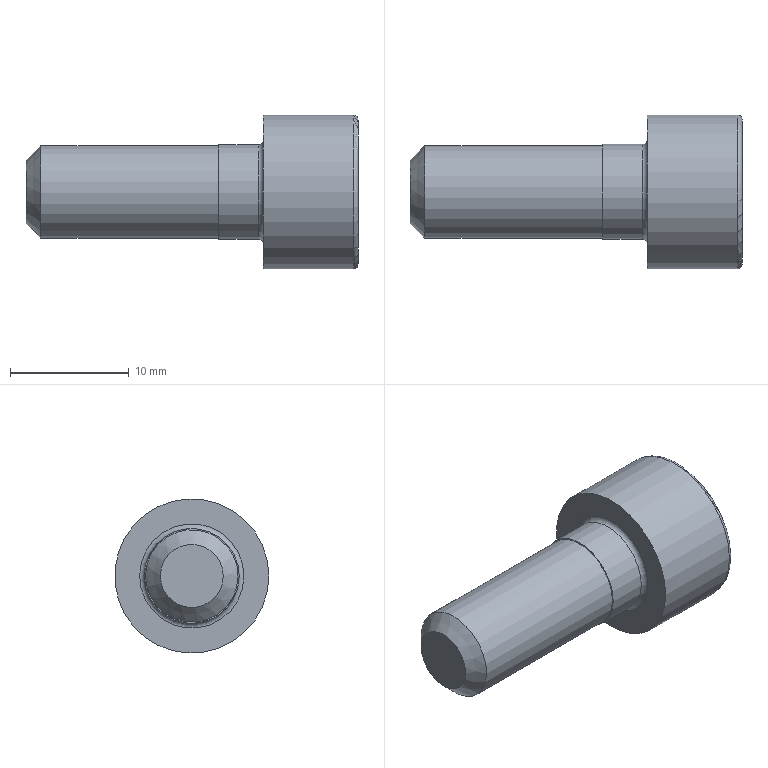Part | STEP file | ISO 4762 SCREW M8x20 STEEL HEXAGON SOCKET HEAD CAP | 1 solid | 24 faces | box 28 x 13 x 13 mm | volume 1862 mm3 | plane 11 | cylinder 9 | torus 2 | cone 2 | commonest cylinder face diameters 6.863 x6 7.805 x1 8 x1 13 x1